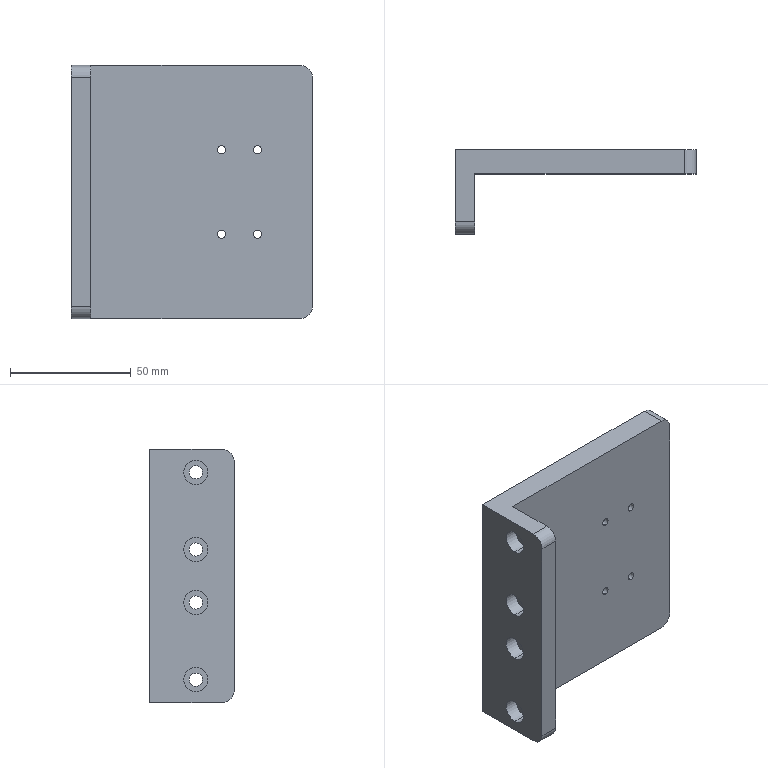Part | SolidWorks | features ICE 5, 3DProfileFeature 2, Fillet 2, HoleWzd 2, ExtruThin 1 | 1 solid | 40 faces | box 100 x 35 x 105 mm | volume 123455 mm3 | cylinder 28 | plane 12 | commonest cylinder face diameters 10 x12 3.3 x8 5.5 x8
STEP:
#1=CARTESIAN_POINT('',(-4.3,-19.1,-48.));
#2=VERTEX_POINT('',#1);
#3=CARTESIAN_POINT('',(-4.3,-19.1,-38.));
#4=VERTEX_POINT('',#3);
#5=CARTESIAN_POINT('',(-4.3,-19.1,-43.));
#6=DIRECTION('',(-1.,0.,0.));
#7=DIRECTION('',(0.,0.,1.));
#8=AXIS2_PLACEMENT_3D('',#5,#6,#7);
#9=CIRCLE('',#8,5.);
#10=EDGE_CURVE('',#2,#4,#9,.T.);
#11=ORIENTED_EDGE('',*,*,#10,.F.);
#12=CARTESIAN_POINT('',(-10.,-19.1,-48.));
#13=VERTEX_POINT('',#12);
#14=CARTESIAN_POINT('',(-10.,-19.1,-48.));
#15=DIRECTION('',(-1.,0.,0.));
#16=VECTOR('',#15,1000.);
#17=LINE('',#14,#16);
#18=EDGE_CURVE('',#2,#13,#17,.T.);
#19=ORIENTED_EDGE('',*,*,#18,.T.);
#20=CARTESIAN_POINT('',(-10.,-19.1,-38.));
#21=VERTEX_POINT('',#20);
#22=CARTESIAN_POINT('',(-10.,-19.1,-43.));
#23=DIRECTION('',(-1.,0.,0.));
#24=DIRECTION('',(0.,0.,1.));
#25=AXIS2_PLACEMENT_3D('',#22,#23,#24);
#26=CIRCLE('',#25,5.);
#27=EDGE_CURVE('',#13,#21,#26,.T.);
#28=ORIENTED_EDGE('',*,*,#27,.T.);
#29=CARTESIAN_POINT('',(-10.,-19.1,-38.));
#30=DIRECTION('',(-1.,0.,0.));
#31=VECTOR('',#30,1000.);
#32=LINE('',#29,#31);
#33=EDGE_CURVE('',#4,#21,#32,.T.);
#34=ORIENTED_EDGE('',*,*,#33,.F.);
#35=EDGE_LOOP('',(#11,#19,#28,#34));
#36=FACE_OUTER_BOUND('',#35,.T.);
#37=CARTESIAN_POINT('',(-10.,-19.1,-43.));
#38=DIRECTION('',(-1.,0.,0.));
#39=DIRECTION('',(0.,0.,1.));
#40=AXIS2_PLACEMENT_3D('',#37,#38,#39);
#41=CYLINDRICAL_SURFACE('',#40,5.);
#42=ADVANCED_FACE('',(#36),#41,.F.);
#43=CARTESIAN_POINT('',(-2.,-19.1,-45.75));
#44=VERTEX_POINT('',#43);
#45=CARTESIAN_POINT('',(-2.,-19.1,-40.25));
#46=VERTEX_POINT('',#45);
#47=CARTESIAN_POINT('',(-2.,-19.1,-43.));
#48=DIRECTION('',(-1.,0.,0.));
#49=DIRECTION('',(0.,0.,1.));
#50=AXIS2_PLACEMENT_3D('',#47,#48,#49);
#51=CIRCLE('',#50,2.75);
#52=EDGE_CURVE('',#44,#46,#51,.T.);
#53=ORIENTED_EDGE('',*,*,#52,.F.);
#54=CARTESIAN_POINT('',(-4.3,-19.1,-45.75));
#55=VERTEX_POINT('',#54);
#56=CARTESIAN_POINT('',(-10.,-19.1,-45.75));
#57=DIRECTION('',(-1.,0.,0.));
#58=VECTOR('',#57,1000.);
#59=LINE('',#56,#58);
#60=EDGE_CURVE('',#44,#55,#59,.T.);
#61=ORIENTED_EDGE('',*,*,#60,.T.);
#62=CARTESIAN_POINT('',(-4.3,-19.1,-40.25));
#63=VERTEX_POINT('',#62);
#64=CARTESIAN_POINT('',(-4.3,-19.1,-43.));
#65=DIRECTION('',(-1.,0.,0.));
#66=DIRECTION('',(0.,0.,1.));
#67=AXIS2_PLACEMENT_3D('',#64,#65,#66);
#68=CIRCLE('',#67,2.75);
#69=EDGE_CURVE('',#55,#63,#68,.T.);
#70=ORIENTED_EDGE('',*,*,#69,.T.);
#71=CARTESIAN_POINT('',(-10.,-19.1,-40.25));
#72=DIRECTION('',(-1.,0.,0.));
#73=VECTOR('',#72,1000.);
#74=LINE('',#71,#73);
#75=EDGE_CURVE('',#46,#63,#74,.T.);
#76=ORIENTED_EDGE('',*,*,#75,.F.);
#77=EDGE_LOOP('',(#53,#61,#70,#76));
#78=FACE_OUTER_BOUND('',#77,.T.);
#79=CARTESIAN_POINT('',(-10.,-19.1,-43.));
#80=DIRECTION('',(-1.,0.,0.));
#81=DIRECTION('',(0.,0.,1.));
#82=AXIS2_PLACEMENT_3D('',#79,#80,#81);
#83=CYLINDRICAL_SURFACE('',#82,2.75);
#84=ADVANCED_FACE('',(#78),#83,.F.);
#85=CARTESIAN_POINT('',(-4.3,-19.1,-16.));
#86=VERTEX_POINT('',#85);
#87=CARTESIAN_POINT('',(-4.3,-19.1,-6.));
#88=VERTEX_POINT('',#87);
#89=CARTESIAN_POINT('',(-4.3,-19.1,-11.));
#90=DIRECTION('',(-1.,0.,0.));
#91=DIRECTION('',(0.,0.,1.));
#92=AXIS2_PLACEMENT_3D('',#89,#90,#91);
#93=CIRCLE('',#92,5.);
#94=EDGE_CURVE('',#86,#88,#93,.T.);
#95=ORIENTED_EDGE('',*,*,#94,.F.);
#96=CARTESIAN_POINT('',(-10.,-19.1,-16.));
#97=VERTEX_POINT('',#96);
#98=CARTESIAN_POINT('',(-10.,-19.1,-16.));
#99=DIRECTION('',(-1.,0.,0.));
#100=VECTOR('',#99,1000.);
#101=LINE('',#98,#100);
#102=EDGE_CURVE('',#86,#97,#101,.T.);
#103=ORIENTED_EDGE('',*,*,#102,.T.);
#104=CARTESIAN_POINT('',(-10.,-19.1,-6.));
#105=VERTEX_POINT('',#104);
#106=CARTESIAN_POINT('',(-10.,-19.1,-11.));
#107=DIRECTION('',(-1.,0.,0.));
#108=DIRECTION('',(0.,0.,1.));
#109=AXIS2_PLACEMENT_3D('',#106,#107,#108);
#110=CIRCLE('',#109,5.);
#111=EDGE_CURVE('',#97,#105,#110,.T.);
#112=ORIENTED_EDGE('',*,*,#111,.T.);
#113=CARTESIAN_POINT('',(-10.,-19.1,-6.));
#114=DIRECTION('',(-1.,0.,0.));
#115=VECTOR('',#114,1000.);
#116=LINE('',#113,#115);
#117=EDGE_CURVE('',#88,#105,#116,.T.);
#118=ORIENTED_EDGE('',*,*,#117,.F.);
#119=EDGE_LOOP('',(#95,#103,#112,#118));
#120=FACE_OUTER_BOUND('',#119,.T.);
#121=CARTESIAN_POINT('',(-10.,-19.1,-11.));
#122=DIRECTION('',(-1.,0.,0.));
#123=DIRECTION('',(0.,0.,1.));
#124=AXIS2_PLACEMENT_3D('',#121,#122,#123);
#125=CYLINDRICAL_SURFACE('',#124,5.);
#126=ADVANCED_FACE('',(#120),#125,.F.);
#127=CARTESIAN_POINT('',(-2.,-19.1,-13.75));
#128=VERTEX_POINT('',#127);
#129=CARTESIAN_POINT('',(-2.,-19.1,-8.25));
#130=VERTEX_POINT('',#129);
#131=CARTESIAN_POINT('',(-2.,-19.1,-11.));
#132=DIRECTION('',(-1.,0.,0.));
#133=DIRECTION('',(0.,0.,1.));
#134=AXIS2_PLACEMENT_3D('',#131,#132,#133);
#135=CIRCLE('',#134,2.75);
#136=EDGE_CURVE('',#128,#130,#135,.T.);
#137=ORIENTED_EDGE('',*,*,#136,.F.);
#138=CARTESIAN_POINT('',(-4.3,-19.1,-13.75));
#139=VERTEX_POINT('',#138);
#140=CARTESIAN_POINT('',(-10.,-19.1,-13.75));
#141=DIRECTION('',(-1.,0.,0.));
#142=VECTOR('',#141,1000.);
#143=LINE('',#140,#142);
#144=EDGE_CURVE('',#128,#139,#143,.T.);
#145=ORIENTED_EDGE('',*,*,#144,.T.);
#146=CARTESIAN_POINT('',(-4.3,-19.1,-8.25));
#147=VERTEX_POINT('',#146);
#148=CARTESIAN_POINT('',(-4.3,-19.1,-11.));
#149=DIRECTION('',(-1.,0.,0.));
#150=DIRECTION('',(0.,0.,1.));
#151=AXIS2_PLACEMENT_3D('',#148,#149,#150);
#152=CIRCLE('',#151,2.75);
#153=EDGE_CURVE('',#139,#147,#152,.T.);
#154=ORIENTED_EDGE('',*,*,#153,.T.);
#155=CARTESIAN_POINT('',(-10.,-19.1,-8.25));
#156=DIRECTION('',(-1.,0.,0.));
#157=VECTOR('',#156,1000.);
#158=LINE('',#155,#157);
#159=EDGE_CURVE('',#130,#147,#158,.T.);
#160=ORIENTED_EDGE('',*,*,#159,.F.);
#161=EDGE_LOOP('',(#137,#145,#154,#160));
#162=FACE_OUTER_BOUND('',#161,.T.);
#163=CARTESIAN_POINT('',(-10.,-19.1,-11.));
#164=DIRECTION('',(-1.,0.,0.));
#165=DIRECTION('',(0.,0.,1.));
#166=AXIS2_PLACEMENT_3D('',#163,#164,#165);
#167=CYLINDRICAL_SURFACE('',#166,2.75);
#168=ADVANCED_FACE('',(#162),#167,.F.);
#169=CARTESIAN_POINT('',(-4.3,-19.1,6.));
#170=VERTEX_POINT('',#169);
#171=CARTESIAN_POINT('',(-4.3,-19.1,16.));
#172=VERTEX_POINT('',#171);
#173=CARTESIAN_POINT('',(-4.3,-19.1,11.));
#174=DIRECTION('',(-1.,0.,0.));
#175=DIRECTION('',(0.,0.,1.));
#176=AXIS2_PLACEMENT_3D('',#173,#174,#175);
#177=CIRCLE('',#176,5.);
#178=EDGE_CURVE('',#170,#172,#177,.T.);
#179=ORIENTED_EDGE('',*,*,#178,.F.);
#180=CARTESIAN_POINT('',(-10.,-19.1,6.));
#181=VERTEX_POINT('',#180);
#182=CARTESIAN_POINT('',(-10.,-19.1,6.));
#183=DIRECTION('',(-1.,0.,0.));
#184=VECTOR('',#183,1000.);
#185=LINE('',#182,#184);
#186=EDGE_CURVE('',#170,#181,#185,.T.);
#187=ORIENTED_EDGE('',*,*,#186,.T.);
#188=CARTESIAN_POINT('',(-10.,-19.1,16.));
#189=VERTEX_POINT('',#188);
#190=CARTESIAN_POINT('',(-10.,-19.1,11.));
#191=DIRECTION('',(-1.,0.,0.));
#192=DIRECTION('',(0.,0.,1.));
#193=AXIS2_PLACEMENT_3D('',#190,#191,#192);
#194=CIRCLE('',#193,5.);
#195=EDGE_CURVE('',#181,#189,#194,.T.);
#196=ORIENTED_EDGE('',*,*,#195,.T.);
#197=CARTESIAN_POINT('',(-10.,-19.1,16.));
#198=DIRECTION('',(-1.,0.,0.));
#199=VECTOR('',#198,1000.);
#200=LINE('',#197,#199);
#201=EDGE_CURVE('',#172,#189,#200,.T.);
#202=ORIENTED_EDGE('',*,*,#201,.F.);
#203=EDGE_LOOP('',(#179,#187,#196,#202));
#204=FACE_OUTER_BOUND('',#203,.T.);
#205=CARTESIAN_POINT('',(-10.,-19.1,11.));
#206=DIRECTION('',(-1.,0.,0.));
#207=DIRECTION('',(0.,0.,1.));
#208=AXIS2_PLACEMENT_3D('',#205,#206,#207);
#209=CYLINDRICAL_SURFACE('',#208,5.);
#210=ADVANCED_FACE('',(#204),#209,.F.);
#211=CARTESIAN_POINT('',(-2.,-19.1,8.25));
#212=VERTEX_POINT('',#211);
#213=CARTESIAN_POINT('',(-2.,-19.1,13.75));
#214=VERTEX_POINT('',#213);
#215=CARTESIAN_POINT('',(-2.,-19.1,11.));
#216=DIRECTION('',(-1.,0.,0.));
#217=DIRECTION('',(0.,0.,1.));
#218=AXIS2_PLACEMENT_3D('',#215,#216,#217);
#219=CIRCLE('',#218,2.75);
#220=EDGE_CURVE('',#212,#214,#219,.T.);
#221=ORIENTED_EDGE('',*,*,#220,.F.);
#222=CARTESIAN_POINT('',(-4.3,-19.1,8.25));
#223=VERTEX_POINT('',#222);
#224=CARTESIAN_POINT('',(-10.,-19.1,8.25));
#225=DIRECTION('',(-1.,0.,0.));
#226=VECTOR('',#225,1000.);
#227=LINE('',#224,#226);
#228=EDGE_CURVE('',#212,#223,#227,.T.);
#229=ORIENTED_EDGE('',*,*,#228,.T.);
#230=CARTESIAN_POINT('',(-4.3,-19.1,13.75));
#231=VERTEX_POINT('',#230);
#232=CARTESIAN_POINT('',(-4.3,-19.1,11.));
#233=DIRECTION('',(-1.,0.,0.));
#234=DIRECTION('',(0.,0.,1.));
#235=AXIS2_PLACEMENT_3D('',#232,#233,#234);
#236=CIRCLE('',#235,2.75);
#237=EDGE_CURVE('',#223,#231,#236,.T.);
#238=ORIENTED_EDGE('',*,*,#237,.T.);
#239=CARTESIAN_POINT('',(-10.,-19.1,13.75));
#240=DIRECTION('',(-1.,0.,0.));
#241=VECTOR('',#240,1000.);
#242=LINE('',#239,#241);
#243=EDGE_CURVE('',#214,#231,#242,.T.);
#244=ORIENTED_EDGE('',*,*,#243,.F.);
#245=EDGE_LOOP('',(#221,#229,#238,#244));
#246=FACE_OUTER_BOUND('',#245,.T.);
#247=CARTESIAN_POINT('',(-10.,-19.1,11.));
#248=DIRECTION('',(-1.,0.,0.));
#249=DIRECTION('',(0.,0.,1.));
#250=AXIS2_PLACEMENT_3D('',#247,#248,#249);
#251=CYLINDRICAL_SURFACE('',#250,2.75);
#252=ADVANCED_FACE('',(#246),#251,.F.);
#253=CARTESIAN_POINT('',(-4.3,-19.1,38.));
#254=VERTEX_POINT('',#253);
#255=CARTESIAN_POINT('',(-4.3,-19.1,48.));
#256=VERTEX_POINT('',#255);
#257=CARTESIAN_POINT('',(-4.3,-19.1,43.));
#258=DIRECTION('',(-1.,0.,0.));
#259=DIRECTION('',(0.,0.,1.));
#260=AXIS2_PLACEMENT_3D('',#257,#258,#259);
#261=CIRCLE('',#260,5.);
#262=EDGE_CURVE('',#254,#256,#261,.T.);
#263=ORIENTED_EDGE('',*,*,#262,.F.);
#264=CARTESIAN_POINT('',(-10.,-19.1,38.));
#265=VERTEX_POINT('',#264);
#266=CARTESIAN_POINT('',(-10.,-19.1,38.));
#267=DIRECTION('',(-1.,0.,0.));
#268=VECTOR('',#267,1000.);
#269=LINE('',#266,#268);
#270=EDGE_CURVE('',#254,#265,#269,.T.);
#271=ORIENTED_EDGE('',*,*,#270,.T.);
#272=CARTESIAN_POINT('',(-10.,-19.1,48.));
#273=VERTEX_POINT('',#272);
#274=CARTESIAN_POINT('',(-10.,-19.1,43.));
#275=DIRECTION('',(-1.,0.,0.));
#276=DIRECTION('',(0.,0.,1.));
#277=AXIS2_PLACEMENT_3D('',#274,#275,#276);
#278=CIRCLE('',#277,5.);
#279=EDGE_CURVE('',#265,#273,#278,.T.);
#280=ORIENTED_EDGE('',*,*,#279,.T.);
#281=CARTESIAN_POINT('',(-10.,-19.1,48.));
#282=DIRECTION('',(-1.,0.,0.));
#283=VECTOR('',#282,1000.);
#284=LINE('',#281,#283);
#285=EDGE_CURVE('',#256,#273,#284,.T.);
#286=ORIENTED_EDGE('',*,*,#285,.F.);
#287=EDGE_LOOP('',(#263,#271,#280,#286));
#288=FACE_OUTER_BOUND('',#287,.T.);
#289=CARTESIAN_POINT('',(-10.,-19.1,43.));
#290=DIRECTION('',(-1.,0.,0.));
#291=DIRECTION('',(0.,0.,1.));
#292=AXIS2_PLACEMENT_3D('',#289,#290,#291);
#293=CYLINDRICAL_SURFACE('',#292,5.);
#294=ADVANCED_FACE('',(#288),#293,.F.);
#295=CARTESIAN_POINT('',(-2.,-19.1,40.25));
#296=VERTEX_POINT('',#295);
#297=CARTESIAN_POINT('',(-2.,-19.1,45.75));
#298=VERTEX_POINT('',#297);
#299=CARTESIAN_POINT('',(-2.,-19.1,43.));
#300=DIRECTION('',(-1.,0.,0.));
#301=DIRECTION('',(0.,0.,1.));
#302=AXIS2_PLACEMENT_3D('',#299,#300,#301);
#303=CIRCLE('',#302,2.75);
#304=EDGE_CURVE('',#296,#298,#303,.T.);
#305=ORIENTED_EDGE('',*,*,#304,.F.);
#306=CARTESIAN_POINT('',(-4.3,-19.1,40.25));
#307=VERTEX_POINT('',#306);
#308=CARTESIAN_POINT('',(-10.,-19.1,40.25));
#309=DIRECTION('',(-1.,0.,0.));
#310=VECTOR('',#309,1000.);
#311=LINE('',#308,#310);
#312=EDGE_CURVE('',#296,#307,#311,.T.);
#313=ORIENTED_EDGE('',*,*,#312,.T.);
#314=CARTESIAN_POINT('',(-4.3,-19.1,45.75));
#315=VERTEX_POINT('',#314);
#316=CARTESIAN_POINT('',(-4.3,-19.1,43.));
#317=DIRECTION('',(-1.,0.,0.));
#318=DIRECTION('',(0.,0.,1.));
#319=AXIS2_PLACEMENT_3D('',#316,#317,#318);
#320=CIRCLE('',#319,2.75);
#321=EDGE_CURVE('',#307,#315,#320,.T.);
#322=ORIENTED_EDGE('',*,*,#321,.T.);
#323=CARTESIAN_POINT('',(-10.,-19.1,45.75));
#324=DIRECTION('',(-1.,0.,0.));
#325=VECTOR('',#324,1000.);
#326=LINE('',#323,#325);
#327=EDGE_CURVE('',#298,#315,#326,.T.);
#328=ORIENTED_EDGE('',*,*,#327,.F.);
#329=EDGE_LOOP('',(#305,#313,#322,#328));
#330=FACE_OUTER_BOUND('',#329,.T.);
#331=CARTESIAN_POINT('',(-10.,-19.1,43.));
#332=DIRECTION('',(-1.,0.,0.));
#333=DIRECTION('',(0.,0.,1.));
#334=AXIS2_PLACEMENT_3D('',#331,#332,#333);
#335=CYLINDRICAL_SURFACE('',#334,2.75);
#336=ADVANCED_FACE('',(#330),#335,.F.);
#337=CARTESIAN_POINT('',(67.2,-10.,15.85));
#338=VERTEX_POINT('',#337);
#339=CARTESIAN_POINT('',(67.2,-10.,19.15));
#340=VERTEX_POINT('',#339);
#341=CARTESIAN_POINT('',(67.2,-10.,17.5));
#342=DIRECTION('',(0.,1.,0.));
#343=DIRECTION('',(0.,0.,1.));
#344=AXIS2_PLACEMENT_3D('',#341,#342,#343);
#345=CIRCLE('',#344,1.65);
#346=EDGE_CURVE('',#338,#340,#345,.T.);
#347=ORIENTED_EDGE('',*,*,#346,.F.);
#348=CARTESIAN_POINT('',(67.2,0.,15.85));
#349=VERTEX_POINT('',#348);
#350=CARTESIAN_POINT('',(67.2,0.,15.85));
#351=DIRECTION('',(0.,1.,0.));
#352=VECTOR('',#351,1000.);
#353=LINE('',#350,#352);
#354=EDGE_CURVE('',#338,#349,#353,.T.);
#355=ORIENTED_EDGE('',*,*,#354,.T.);
#356=CARTESIAN_POINT('',(67.2,0.,19.15));
#357=VERTEX_POINT('',#356);
#358=CARTESIAN_POINT('',(67.2,0.,17.5));
#359=DIRECTION('',(0.,1.,0.));
#360=DIRECTION('',(0.,0.,1.));
#361=AXIS2_PLACEMENT_3D('',#358,#359,#360);
#362=CIRCLE('',#361,1.65);
#363=EDGE_CURVE('',#349,#357,#362,.T.);
#364=ORIENTED_EDGE('',*,*,#363,.T.);
#365=CARTESIAN_POINT('',(67.2,0.,19.15));
#366=DIRECTION('',(0.,1.,0.));
#367=VECTOR('',#366,1000.);
#368=LINE('',#365,#367);
#369=EDGE_CURVE('',#340,#357,#368,.T.);
#370=ORIENTED_EDGE('',*,*,#369,.F.);
#371=EDGE_LOOP('',(#347,#355,#364,#370));
#372=FACE_OUTER_BOUND('',#371,.T.);
#373=CARTESIAN_POINT('',(67.2,0.,17.5));
#374=DIRECTION('',(0.,1.,0.));
#375=DIRECTION('',(0.,0.,1.));
#376=AXIS2_PLACEMENT_3D('',#373,#374,#375);
#377=CYLINDRICAL_SURFACE('',#376,1.65);
#378=ADVANCED_FACE('',(#372),#377,.F.);
#379=CARTESIAN_POINT('',(52.2,-10.,15.85));
#380=VERTEX_POINT('',#379);
#381=CARTESIAN_POINT('',(52.2,-10.,19.15));
#382=VERTEX_POINT('',#381);
#383=CARTESIAN_POINT('',(52.2,-10.,17.5));
#384=DIRECTION('',(0.,1.,0.));
#385=DIRECTION('',(0.,0.,1.));
#386=AXIS2_PLACEMENT_3D('',#383,#384,#385);
#387=CIRCLE('',#386,1.65);
#388=EDGE_CURVE('',#380,#382,#387,.T.);
#389=ORIENTED_EDGE('',*,*,#388,.F.);
#390=CARTESIAN_POINT('',(52.2,0.,15.85));
#391=VERTEX_POINT('',#390);
#392=CARTESIAN_POINT('',(52.2,0.,15.85));
#393=DIRECTION('',(0.,1.,0.));
#394=VECTOR('',#393,1000.);
#395=LINE('',#392,#394);
#396=EDGE_CURVE('',#380,#391,#395,.T.);
#397=ORIENTED_EDGE('',*,*,#396,.T.);
#398=CARTESIAN_POINT('',(52.2,0.,19.15));
#399=VERTEX_POINT('',#398);
#400=CARTESIAN_POINT('',(52.2,0.,17.5));
#401=DIRECTION('',(0.,1.,0.));
#402=DIRECTION('',(0.,0.,1.));
#403=AXIS2_PLACEMENT_3D('',#400,#401,#402);
#404=CIRCLE('',#403,1.65);
#405=EDGE_CURVE('',#391,#399,#404,.T.);
#406=ORIENTED_EDGE('',*,*,#405,.T.);
#407=CARTESIAN_POINT('',(52.2,0.,19.15));
#408=DIRECTION('',(0.,1.,0.));
#409=VECTOR('',#408,1000.);
#410=LINE('',#407,#409);
#411=EDGE_CURVE('',#382,#399,#410,.T.);
#412=ORIENTED_EDGE('',*,*,#411,.F.);
#413=EDGE_LOOP('',(#389,#397,#406,#412));
#414=FACE_OUTER_BOUND('',#413,.T.);
#415=CARTESIAN_POINT('',(52.2,0.,17.5));
#416=DIRECTION('',(0.,1.,0.));
#417=DIRECTION('',(0.,0.,1.));
#418=AXIS2_PLACEMENT_3D('',#415,#416,#417);
#419=CYLINDRICAL_SURFACE('',#418,1.65);
#420=ADVANCED_FACE('',(#414),#419,.F.);
#421=CARTESIAN_POINT('',(67.2,-10.,-19.15));
#422=VERTEX_POINT('',#421);
#423=CARTESIAN_POINT('',(67.2,-10.,-15.85));
#424=VERTEX_POINT('',#423);
#425=CARTESIAN_POINT('',(67.2,-10.,-17.5));
#426=DIRECTION('',(0.,1.,0.));
#427=DIRECTION('',(0.,0.,1.));
#428=AXIS2_PLACEMENT_3D('',#425,#426,#427);
#429=CIRCLE('',#428,1.65);
#430=EDGE_CURVE('',#422,#424,#429,.T.);
#431=ORIENTED_EDGE('',*,*,#430,.F.);
#432=CARTESIAN_POINT('',(67.2,0.,-19.15));
#433=VERTEX_POINT('',#432);
#434=CARTESIAN_POINT('',(67.2,0.,-19.15));
#435=DIRECTION('',(0.,1.,0.));
#436=VECTOR('',#435,1000.);
#437=LINE('',#434,#436);
#438=EDGE_CURVE('',#422,#433,#437,.T.);
#439=ORIENTED_EDGE('',*,*,#438,.T.);
#440=CARTESIAN_POINT('',(67.2,0.,-15.85));
#441=VERTEX_POINT('',#440);
#442=CARTESIAN_POINT('',(67.2,0.,-17.5));
#443=DIRECTION('',(0.,1.,0.));
#444=DIRECTION('',(0.,0.,1.));
#445=AXIS2_PLACEMENT_3D('',#442,#443,#444);
#446=CIRCLE('',#445,1.65);
#447=EDGE_CURVE('',#433,#441,#446,.T.);
#448=ORIENTED_EDGE('',*,*,#447,.T.);
#449=CARTESIAN_POINT('',(67.2,0.,-15.85));
#450=DIRECTION('',(0.,1.,0.));
#451=VECTOR('',#450,1000.);
#452=LINE('',#449,#451);
#453=EDGE_CURVE('',#424,#441,#452,.T.);
#454=ORIENTED_EDGE('',*,*,#453,.F.);
#455=EDGE_LOOP('',(#431,#439,#448,#454));
#456=FACE_OUTER_BOUND('',#455,.T.);
#457=CARTESIAN_POINT('',(67.2,0.,-17.5));
#458=DIRECTION('',(0.,1.,0.));
#459=DIRECTION('',(0.,0.,1.));
#460=AXIS2_PLACEMENT_3D('',#457,#458,#459);
#461=CYLINDRICAL_SURFACE('',#460,1.65);
#462=ADVANCED_FACE('',(#456),#461,.F.);
#463=CARTESIAN_POINT('',(52.2,-10.,-19.15));
#464=VERTEX_POINT('',#463);
#465=CARTESIAN_POINT('',(52.2,-10.,-15.85));
#466=VERTEX_POINT('',#465);
#467=CARTESIAN_POINT('',(52.2,-10.,-17.5));
#468=DIRECTION('',(0.,1.,0.));
#469=DIRECTION('',(0.,0.,1.));
#470=AXIS2_PLACEMENT_3D('',#467,#468,#469);
#471=CIRCLE('',#470,1.65);
#472=EDGE_CURVE('',#464,#466,#471,.T.);
#473=ORIENTED_EDGE('',*,*,#472,.F.);
#474=CARTESIAN_POINT('',(52.2,0.,-19.15));
#475=VERTEX_POINT('',#474);
#476=CARTESIAN_POINT('',(52.2,0.,-19.15));
#477=DIRECTION('',(0.,1.,0.));
#478=VECTOR('',#477,1000.);
#479=LINE('',#476,#478);
#480=EDGE_CURVE('',#464,#475,#479,.T.);
#481=ORIENTED_EDGE('',*,*,#480,.T.);
#482=CARTESIAN_POINT('',(52.2,0.,-15.85));
#483=VERTEX_POINT('',#482);
#484=CARTESIAN_POINT('',(52.2,0.,-17.5));
#485=DIRECTION('',(0.,1.,0.));
#486=DIRECTION('',(0.,0.,1.));
#487=AXIS2_PLACEMENT_3D('',#484,#485,#486);
#488=CIRCLE('',#487,1.65);
#489=EDGE_CURVE('',#475,#483,#488,.T.);
#490=ORIENTED_EDGE('',*,*,#489,.T.);
#491=CARTESIAN_POINT('',(52.2,0.,-15.85));
#492=DIRECTION('',(0.,1.,0.));
#493=VECTOR('',#492,1000.);
#494=LINE('',#491,#493);
#495=EDGE_CURVE('',#466,#483,#494,.T.);
#496=ORIENTED_EDGE('',*,*,#495,.F.);
#497=EDGE_LOOP('',(#473,#481,#490,#496));
#498=FACE_OUTER_BOUND('',#497,.T.);
#499=CARTESIAN_POINT('',(52.2,0.,-17.5));
#500=DIRECTION('',(0.,1.,0.));
#501=DIRECTION('',(0.,0.,1.));
#502=AXIS2_PLACEMENT_3D('',#499,#500,#501);
#503=CYLINDRICAL_SURFACE('',#502,1.65);
#504=ADVANCED_FACE('',(#498),#503,.F.);
#505=CARTESIAN_POINT('',(-10.,-19.1,-11.));
#506=DIRECTION('',(-1.,0.,0.));
#507=DIRECTION('',(0.,0.,1.));
#508=AXIS2_PLACEMENT_3D('',#505,#506,#507);
#509=CIRCLE('',#508,5.);
#510=EDGE_CURVE('',#105,#97,#509,.T.);
#511=ORIENTED_EDGE('',*,*,#510,.F.);
#512=ORIENTED_EDGE('',*,*,#111,.F.);
#513=EDGE_LOOP('',(#511,#512));
#514=FACE_BOUND('',#513,.T.);
#515=CARTESIAN_POINT('',(-10.,-19.1,11.));
#516=DIRECTION('',(-1.,0.,0.));
#517=DIRECTION('',(0.,0.,1.));
#518=AXIS2_PLACEMENT_3D('',#515,#516,#517);
#519=CIRCLE('',#518,5.);
#520=EDGE_CURVE('',#189,#181,#519,.T.);
#521=ORIENTED_EDGE('',*,*,#520,.F.);
#522=ORIENTED_EDGE('',*,*,#195,.F.);
#523=EDGE_LOOP('',(#521,#522));
#524=FACE_BOUND('',#523,.T.);
#525=CARTESIAN_POINT('',(-10.,-19.1,43.));
#526=DIRECTION('',(-1.,0.,0.));
#527=DIRECTION('',(0.,0.,1.));
#528=AXIS2_PLACEMENT_3D('',#525,#526,#527);
#529=CIRCLE('',#528,5.);
#530=EDGE_CURVE('',#273,#265,#529,.T.);
#531=ORIENTED_EDGE('',*,*,#530,.F.);
#532=ORIENTED_EDGE('',*,*,#279,.F.);
#533=EDGE_LOOP('',(#531,#532));
#534=FACE_BOUND('',#533,.T.);
#535=CARTESIAN_POINT('',(-10.,-30.,-52.5));
#536=VERTEX_POINT('',#535);
#537=CARTESIAN_POINT('',(-10.,0.,-52.5));
#538=VERTEX_POINT('',#537);
#539=CARTESIAN_POINT('',(-10.,-155.,-52.5));
#540=DIRECTION('',(0.,1.,0.));
#541=VECTOR('',#540,1000.);
#542=LINE('',#539,#541);
#543=EDGE_CURVE('',#536,#538,#542,.T.);
#544=ORIENTED_EDGE('',*,*,#543,.F.);
#545=CARTESIAN_POINT('',(-10.,-35.,-47.5));
#546=VERTEX_POINT('',#545);
#547=CARTESIAN_POINT('',(-10.,-30.,-47.5));
#548=DIRECTION('',(-1.,0.,0.));
#549=DIRECTION('',(0.,0.,-1.));
#550=AXIS2_PLACEMENT_3D('',#547,#548,#549);
#551=CIRCLE('',#550,5.);
#552=EDGE_CURVE('',#536,#546,#551,.T.);
#553=ORIENTED_EDGE('',*,*,#552,.T.);
#554=CARTESIAN_POINT('',(-10.,-35.,47.5));
#555=VERTEX_POINT('',#554);
#556=CARTESIAN_POINT('',(-10.,-35.,-52.5));
#557=DIRECTION('',(0.,0.,1.));
#558=VECTOR('',#557,1000.);
#559=LINE('',#556,#558);
#560=EDGE_CURVE('',#546,#555,#559,.T.);
#561=ORIENTED_EDGE('',*,*,#560,.T.);
#562=CARTESIAN_POINT('',(-10.,-30.,52.5));
#563=VERTEX_POINT('',#562);
#564=CARTESIAN_POINT('',(-10.,-30.,47.5));
#565=DIRECTION('',(-1.,0.,0.));
#566=DIRECTION('',(0.,0.,-1.));
#567=AXIS2_PLACEMENT_3D('',#564,#565,#566);
#568=CIRCLE('',#567,5.);
#569=EDGE_CURVE('',#555,#563,#568,.T.);
#570=ORIENTED_EDGE('',*,*,#569,.T.);
#571=CARTESIAN_POINT('',(-10.,0.,52.5));
#572=VERTEX_POINT('',#571);
#573=CARTESIAN_POINT('',(-10.,-155.,52.5));
#574=DIRECTION('',(0.,1.,0.));
#575=VECTOR('',#574,1000.);
#576=LINE('',#573,#575);
#577=EDGE_CURVE('',#563,#572,#576,.T.);
#578=ORIENTED_EDGE('',*,*,#577,.T.);
#579=CARTESIAN_POINT('',(-10.,0.,52.5));
#580=DIRECTION('',(0.,0.,1.));
#581=VECTOR('',#580,1000.);
#582=LINE('',#579,#581);
#583=EDGE_CURVE('',#538,#572,#582,.T.);
#584=ORIENTED_EDGE('',*,*,#583,.F.);
#585=EDGE_LOOP('',(#544,#553,#561,#570,#578,#584));
#586=FACE_OUTER_BOUND('',#585,.T.);
#587=CARTESIAN_POINT('',(-10.,-19.1,-43.));
#588=DIRECTION('',(-1.,0.,0.));
#589=DIRECTION('',(0.,0.,1.));
#590=AXIS2_PLACEMENT_3D('',#587,#588,#589);
#591=CIRCLE('',#590,5.);
#592=EDGE_CURVE('',#21,#13,#591,.T.);
#593=ORIENTED_EDGE('',*,*,#592,.F.);
#594=ORIENTED_EDGE('',*,*,#27,.F.);
#595=EDGE_LOOP('',(#593,#594));
#596=FACE_BOUND('',#595,.T.);
#597=CARTESIAN_POINT('',(-10.,0.,27.));
#598=DIRECTION('',(1.,0.,0.));
#599=DIRECTION('',(0.,0.,-1.));
#600=AXIS2_PLACEMENT_3D('',#597,#598,#599);
#601=PLANE('',#600);
#602=ADVANCED_FACE('',(#514,#524,#534,#586,#596),#601,.F.);
#603=CARTESIAN_POINT('',(52.2,-10.,-17.5));
#604=DIRECTION('',(0.,1.,0.));
#605=DIRECTION('',(0.,0.,1.));
#606=AXIS2_PLACEMENT_3D('',#603,#604,#605);
#607=CIRCLE('',#606,1.65);
#608=EDGE_CURVE('',#466,#464,#607,.T.);
#609=ORIENTED_EDGE('',*,*,#608,.T.);
#610=ORIENTED_EDGE('',*,*,#472,.T.);
#611=EDGE_LOOP('',(#609,#610));
#612=FACE_BOUND('',#611,.T.);
#613=CARTESIAN_POINT('',(67.2,-10.,-17.5));
#614=DIRECTION('',(0.,1.,0.));
#615=DIRECTION('',(0.,0.,1.));
#616=AXIS2_PLACEMENT_3D('',#613,#614,#615);
#617=CIRCLE('',#616,1.65);
#618=EDGE_CURVE('',#424,#422,#617,.T.);
#619=ORIENTED_EDGE('',*,*,#618,.T.);
#620=ORIENTED_EDGE('',*,*,#430,.T.);
#621=EDGE_LOOP('',(#619,#620));
#622=FACE_BOUND('',#621,.T.);
#623=CARTESIAN_POINT('',(52.2,-10.,17.5));
#624=DIRECTION('',(0.,1.,0.));
#625=DIRECTION('',(0.,0.,1.));
#626=AXIS2_PLACEMENT_3D('',#623,#624,#625);
#627=CIRCLE('',#626,1.65);
#628=EDGE_CURVE('',#382,#380,#627,.T.);
#629=ORIENTED_EDGE('',*,*,#628,.T.);
#630=ORIENTED_EDGE('',*,*,#388,.T.);
#631=EDGE_LOOP('',(#629,#630));
#632=FACE_BOUND('',#631,.T.);
#633=CARTESIAN_POINT('',(67.2,-10.,17.5));
#634=DIRECTION('',(0.,1.,0.));
#635=DIRECTION('',(0.,0.,1.));
#636=AXIS2_PLACEMENT_3D('',#633,#634,#635);
#637=CIRCLE('',#636,1.65);
#638=EDGE_CURVE('',#340,#338,#637,.T.);
#639=ORIENTED_EDGE('',*,*,#638,.T.);
#640=ORIENTED_EDGE('',*,*,#346,.T.);
#641=EDGE_LOOP('',(#639,#640));
#642=FACE_BOUND('',#641,.T.);
#643=CARTESIAN_POINT('',(-2.,-10.,-52.5));
#644=VERTEX_POINT('',#643);
#645=CARTESIAN_POINT('',(-2.,-10.,52.5));
#646=VERTEX_POINT('',#645);
#647=CARTESIAN_POINT('',(-2.,-10.,27.));
#648=DIRECTION('',(0.,0.,1.));
#649=VECTOR('',#648,1000.);
#650=LINE('',#647,#649);
#651=EDGE_CURVE('',#644,#646,#650,.T.);
#652=ORIENTED_EDGE('',*,*,#651,.F.);
#653=CARTESIAN_POINT('',(85.,-10.,-52.5));
#654=VERTEX_POINT('',#653);
#655=CARTESIAN_POINT('',(-10.,-10.,-52.5));
#656=DIRECTION('',(1.,0.,0.));
#657=VECTOR('',#656,1000.);
#658=LINE('',#655,#657);
#659=EDGE_CURVE('',#644,#654,#658,.T.);
#660=ORIENTED_EDGE('',*,*,#659,.T.);
#661=CARTESIAN_POINT('',(90.,-10.,-47.5));
#662=VERTEX_POINT('',#661);
#663=CARTESIAN_POINT('',(85.,-10.,-47.5));
#664=DIRECTION('',(0.,-1.,0.));
#665=DIRECTION('',(0.,0.,1.));
#666=AXIS2_PLACEMENT_3D('',#663,#664,#665);
#667=CIRCLE('',#666,5.);
#668=EDGE_CURVE('',#654,#662,#667,.T.);
#669=ORIENTED_EDGE('',*,*,#668,.T.);
#670=CARTESIAN_POINT('',(90.,-10.,47.5));
#671=VERTEX_POINT('',#670);
#672=CARTESIAN_POINT('',(90.,-10.,27.));
#673=DIRECTION('',(0.,0.,-1.));
#674=VECTOR('',#673,1000.);
#675=LINE('',#672,#674);
#676=EDGE_CURVE('',#671,#662,#675,.T.);
#677=ORIENTED_EDGE('',*,*,#676,.F.);
#678=CARTESIAN_POINT('',(85.,-10.,52.5));
#679=VERTEX_POINT('',#678);
#680=CARTESIAN_POINT('',(85.,-10.,47.5));
#681=DIRECTION('',(0.,-1.,0.));
#682=DIRECTION('',(0.,0.,1.));
#683=AXIS2_PLACEMENT_3D('',#680,#681,#682);
#684=CIRCLE('',#683,5.);
#685=EDGE_CURVE('',#671,#679,#684,.T.);
#686=ORIENTED_EDGE('',*,*,#685,.T.);
#687=CARTESIAN_POINT('',(-10.,-10.,52.5));
#688=DIRECTION('',(-1.,0.,0.));
#689=VECTOR('',#688,1000.);
#690=LINE('',#687,#689);
#691=EDGE_CURVE('',#679,#646,#690,.T.);
#692=ORIENTED_EDGE('',*,*,#691,.T.);
#693=EDGE_LOOP('',(#652,#660,#669,#677,#686,#692));
#694=FACE_OUTER_BOUND('',#693,.T.);
#695=CARTESIAN_POINT('',(0.,-10.,27.));
#696=DIRECTION('',(0.,1.,0.));
#697=DIRECTION('',(0.,0.,1.));
#698=AXIS2_PLACEMENT_3D('',#695,#696,#697);
#699=PLANE('',#698);
#700=ADVANCED_FACE('',(#612,#622,#632,#642,#694),#699,.F.);
#701=ORIENTED_EDGE('',*,*,#676,.T.);
#702=CARTESIAN_POINT('',(90.,0.,-47.5));
#703=VERTEX_POINT('',#702);
#704=CARTESIAN_POINT('',(90.,0.,-47.5));
#705=DIRECTION('',(0.,1.,0.));
#706=VECTOR('',#705,1000.);
#707=LINE('',#704,#706);
#708=EDGE_CURVE('',#662,#703,#707,.T.);
#709=ORIENTED_EDGE('',*,*,#708,.T.);
#710=CARTESIAN_POINT('',(90.,0.,47.5));
#711=VERTEX_POINT('',#710);
#712=CARTESIAN_POINT('',(90.,0.,27.));
#713=DIRECTION('',(0.,0.,-1.));
#714=VECTOR('',#713,1000.);
#715=LINE('',#712,#714);
#716=EDGE_CURVE('',#711,#703,#715,.T.);
#717=ORIENTED_EDGE('',*,*,#716,.F.);
#718=CARTESIAN_POINT('',(90.,0.,47.5));
#719=DIRECTION('',(0.,-1.,0.));
#720=VECTOR('',#719,1000.);
#721=LINE('',#718,#720);
#722=EDGE_CURVE('',#711,#671,#721,.T.);
#723=ORIENTED_EDGE('',*,*,#722,.T.);
#724=EDGE_LOOP('',(#701,#709,#717,#723));
#725=FACE_OUTER_BOUND('',#724,.T.);
#726=CARTESIAN_POINT('',(90.,0.,27.));
#727=DIRECTION('',(1.,0.,0.));
#728=DIRECTION('',(0.,0.,-1.));
#729=AXIS2_PLACEMENT_3D('',#726,#727,#728);
#730=PLANE('',#729);
#731=ADVANCED_FACE('',(#725),#730,.T.);
#732=CARTESIAN_POINT('',(85.,0.,52.5));
#733=VERTEX_POINT('',#732);
#734=CARTESIAN_POINT('',(-10.,0.,52.5));
#735=DIRECTION('',(1.,0.,0.));
#736=VECTOR('',#735,1000.);
#737=LINE('',#734,#736);
#738=EDGE_CURVE('',#572,#733,#737,.T.);
#739=ORIENTED_EDGE('',*,*,#738,.T.);
#740=CARTESIAN_POINT('',(85.,0.,47.5));
#741=DIRECTION('',(0.,1.,0.));
#742=DIRECTION('',(0.,0.,1.));
#743=AXIS2_PLACEMENT_3D('',#740,#741,#742);
#744=CIRCLE('',#743,5.);
#745=EDGE_CURVE('',#733,#711,#744,.T.);
#746=ORIENTED_EDGE('',*,*,#745,.T.);
#747=ORIENTED_EDGE('',*,*,#716,.T.);
#748=CARTESIAN_POINT('',(85.,0.,-52.5));
#749=VERTEX_POINT('',#748);
#750=CARTESIAN_POINT('',(85.,0.,-47.5));
#751=DIRECTION('',(0.,1.,0.));
#752=DIRECTION('',(0.,0.,1.));
#753=AXIS2_PLACEMENT_3D('',#750,#751,#752);
#754=CIRCLE('',#753,5.);
#755=EDGE_CURVE('',#703,#749,#754,.T.);
#756=ORIENTED_EDGE('',*,*,#755,.T.);
#757=CARTESIAN_POINT('',(-10.,0.,-52.5));
#758=DIRECTION('',(-1.,0.,0.));
#759=VECTOR('',#758,1000.);
#760=LINE('',#757,#759);
#761=EDGE_CURVE('',#749,#538,#760,.T.);
#762=ORIENTED_EDGE('',*,*,#761,.T.);
#763=ORIENTED_EDGE('',*,*,#583,.T.);
#764=EDGE_LOOP('',(#739,#746,#747,#756,#762,#763));
#765=FACE_OUTER_BOUND('',#764,.T.);
#766=CARTESIAN_POINT('',(67.2,0.,17.5));
#767=DIRECTION('',(0.,1.,0.));
#768=DIRECTION('',(0.,0.,1.));
#769=AXIS2_PLACEMENT_3D('',#766,#767,#768);
#770=CIRCLE('',#769,1.65);
#771=EDGE_CURVE('',#357,#349,#770,.T.);
#772=ORIENTED_EDGE('',*,*,#771,.F.);
#773=ORIENTED_EDGE('',*,*,#363,.F.);
#774=EDGE_LOOP('',(#772,#773));
#775=FACE_BOUND('',#774,.T.);
#776=CARTESIAN_POINT('',(52.2,0.,17.5));
#777=DIRECTION('',(0.,1.,0.));
#778=DIRECTION('',(0.,0.,1.));
#779=AXIS2_PLACEMENT_3D('',#776,#777,#778);
#780=CIRCLE('',#779,1.65);
#781=EDGE_CURVE('',#399,#391,#780,.T.);
#782=ORIENTED_EDGE('',*,*,#781,.F.);
#783=ORIENTED_EDGE('',*,*,#405,.F.);
#784=EDGE_LOOP('',(#782,#783));
#785=FACE_BOUND('',#784,.T.);
#786=CARTESIAN_POINT('',(67.2,0.,-17.5));
#787=DIRECTION('',(0.,1.,0.));
#788=DIRECTION('',(0.,0.,1.));
#789=AXIS2_PLACEMENT_3D('',#786,#787,#788);
#790=CIRCLE('',#789,1.65);
#791=EDGE_CURVE('',#441,#433,#790,.T.);
#792=ORIENTED_EDGE('',*,*,#791,.F.);
#793=ORIENTED_EDGE('',*,*,#447,.F.);
#794=EDGE_LOOP('',(#792,#793));
#795=FACE_BOUND('',#794,.T.);
#796=CARTESIAN_POINT('',(52.2,0.,-17.5));
#797=DIRECTION('',(0.,1.,0.));
#798=DIRECTION('',(0.,0.,1.));
#799=AXIS2_PLACEMENT_3D('',#796,#797,#798);
#800=CIRCLE('',#799,1.65);
#801=EDGE_CURVE('',#483,#475,#800,.T.);
#802=ORIENTED_EDGE('',*,*,#801,.F.);
#803=ORIENTED_EDGE('',*,*,#489,.F.);
#804=EDGE_LOOP('',(#802,#803));
#805=FACE_BOUND('',#804,.T.);
#806=CARTESIAN_POINT('',(0.,0.,27.));
#807=DIRECTION('',(0.,1.,0.));
#808=DIRECTION('',(0.,0.,1.));
#809=AXIS2_PLACEMENT_3D('',#806,#807,#808);
#810=PLANE('',#809);
#811=ADVANCED_FACE('',(#765,#775,#785,#795,#805),#810,.T.);
#812=CARTESIAN_POINT('',(-2.,-30.,-52.5));
#813=VERTEX_POINT('',#812);
#814=CARTESIAN_POINT('',(-2.,0.,-52.5));
#815=DIRECTION('',(0.,-1.,0.));
#816=VECTOR('',#815,1000.);
#817=LINE('',#814,#816);
#818=EDGE_CURVE('',#644,#813,#817,.T.);
#819=ORIENTED_EDGE('',*,*,#818,.T.);
#820=CARTESIAN_POINT('',(-10.,-30.,-52.5));
#821=DIRECTION('',(-1.,0.,0.));
#822=VECTOR('',#821,1000.);
#823=LINE('',#820,#822);
#824=EDGE_CURVE('',#813,#536,#823,.T.);
#825=ORIENTED_EDGE('',*,*,#824,.T.);
#826=ORIENTED_EDGE('',*,*,#543,.T.);
#827=ORIENTED_EDGE('',*,*,#761,.F.);
#828=CARTESIAN_POINT('',(85.,-155.,-52.5));
#829=DIRECTION('',(0.,-1.,0.));
#830=VECTOR('',#829,1000.);
#831=LINE('',#828,#830);
#832=EDGE_CURVE('',#749,#654,#831,.T.);
#833=ORIENTED_EDGE('',*,*,#832,.T.);
#834=ORIENTED_EDGE('',*,*,#659,.F.);
#835=EDGE_LOOP('',(#819,#825,#826,#827,#833,#834));
#836=FACE_OUTER_BOUND('',#835,.T.);
#837=CARTESIAN_POINT('',(-10.,-155.,-52.5));
#838=DIRECTION('',(0.,0.,-1.));
#839=DIRECTION('',(-1.,0.,0.));
#840=AXIS2_PLACEMENT_3D('',#837,#838,#839);
#841=PLANE('',#840);
#842=ADVANCED_FACE('',(#836),#841,.T.);
#843=ORIENTED_EDGE('',*,*,#577,.F.);
#844=CARTESIAN_POINT('',(-2.,-30.,52.5));
#845=VERTEX_POINT('',#844);
#846=CARTESIAN_POINT('',(-10.,-30.,52.5));
#847=DIRECTION('',(1.,0.,0.));
#848=VECTOR('',#847,1000.);
#849=LINE('',#846,#848);
#850=EDGE_CURVE('',#563,#845,#849,.T.);
#851=ORIENTED_EDGE('',*,*,#850,.T.);
#852=CARTESIAN_POINT('',(-2.,0.,52.5));
#853=DIRECTION('',(0.,1.,0.));
#854=VECTOR('',#853,1000.);
#855=LINE('',#852,#854);
#856=EDGE_CURVE('',#845,#646,#855,.T.);
#857=ORIENTED_EDGE('',*,*,#856,.T.);
#858=ORIENTED_EDGE('',*,*,#691,.F.);
#859=CARTESIAN_POINT('',(85.,-155.,52.5));
#860=DIRECTION('',(0.,1.,0.));
#861=VECTOR('',#860,1000.);
#862=LINE('',#859,#861);
#863=EDGE_CURVE('',#679,#733,#862,.T.);
#864=ORIENTED_EDGE('',*,*,#863,.T.);
#865=ORIENTED_EDGE('',*,*,#738,.F.);
#866=EDGE_LOOP('',(#843,#851,#857,#858,#864,#865));
#867=FACE_OUTER_BOUND('',#866,.T.);
#868=CARTESIAN_POINT('',(-10.,-155.,52.5));
#869=DIRECTION('',(0.,0.,1.));
#870=DIRECTION('',(1.,0.,0.));
#871=AXIS2_PLACEMENT_3D('',#868,#869,#870);
#872=PLANE('',#871);
#873=ADVANCED_FACE('',(#867),#872,.T.);
#874=ORIENTED_EDGE('',*,*,#668,.F.);
#875=ORIENTED_EDGE('',*,*,#832,.F.);
#876=ORIENTED_EDGE('',*,*,#755,.F.);
#877=ORIENTED_EDGE('',*,*,#708,.F.);
#878=EDGE_LOOP('',(#874,#875,#876,#877));
#879=FACE_OUTER_BOUND('',#878,.T.);
#880=CARTESIAN_POINT('',(85.,0.,-47.5));
#881=DIRECTION('',(0.,1.,0.));
#882=DIRECTION('',(0.,0.,1.));
#883=AXIS2_PLACEMENT_3D('',#880,#881,#882);
#884=CYLINDRICAL_SURFACE('',#883,5.);
#885=ADVANCED_FACE('',(#879),#884,.T.);
#886=ORIENTED_EDGE('',*,*,#685,.F.);
#887=ORIENTED_EDGE('',*,*,#722,.F.);
#888=ORIENTED_EDGE('',*,*,#745,.F.);
#889=ORIENTED_EDGE('',*,*,#863,.F.);
#890=EDGE_LOOP('',(#886,#887,#888,#889));
#891=FACE_OUTER_BOUND('',#890,.T.);
#892=CARTESIAN_POINT('',(85.,-155.,47.5));
#893=DIRECTION('',(0.,1.,0.));
#894=DIRECTION('',(0.,0.,1.));
#895=AXIS2_PLACEMENT_3D('',#892,#893,#894);
#896=CYLINDRICAL_SURFACE('',#895,5.);
#897=ADVANCED_FACE('',(#891),#896,.T.);
#898=ORIENTED_EDGE('',*,*,#480,.F.);
#899=ORIENTED_EDGE('',*,*,#608,.F.);
#900=ORIENTED_EDGE('',*,*,#495,.T.);
#901=ORIENTED_EDGE('',*,*,#801,.T.);
#902=EDGE_LOOP('',(#898,#899,#900,#901));
#903=FACE_OUTER_BOUND('',#902,.T.);
#904=CARTESIAN_POINT('',(52.2,0.,-17.5));
#905=DIRECTION('',(0.,1.,0.));
#906=DIRECTION('',(0.,0.,1.));
#907=AXIS2_PLACEMENT_3D('',#904,#905,#906);
#908=CYLINDRICAL_SURFACE('',#907,1.65);
#909=ADVANCED_FACE('',(#903),#908,.F.);
#910=ORIENTED_EDGE('',*,*,#438,.F.);
#911=ORIENTED_EDGE('',*,*,#618,.F.);
#912=ORIENTED_EDGE('',*,*,#453,.T.);
#913=ORIENTED_EDGE('',*,*,#791,.T.);
#914=EDGE_LOOP('',(#910,#911,#912,#913));
#915=FACE_OUTER_BOUND('',#914,.T.);
#916=CARTESIAN_POINT('',(67.2,0.,-17.5));
#917=DIRECTION('',(0.,1.,0.));
#918=DIRECTION('',(0.,0.,1.));
#919=AXIS2_PLACEMENT_3D('',#916,#917,#918);
#920=CYLINDRICAL_SURFACE('',#919,1.65);
#921=ADVANCED_FACE('',(#915),#920,.F.);
#922=ORIENTED_EDGE('',*,*,#396,.F.);
#923=ORIENTED_EDGE('',*,*,#628,.F.);
#924=ORIENTED_EDGE('',*,*,#411,.T.);
#925=ORIENTED_EDGE('',*,*,#781,.T.);
#926=EDGE_LOOP('',(#922,#923,#924,#925));
#927=FACE_OUTER_BOUND('',#926,.T.);
#928=CARTESIAN_POINT('',(52.2,0.,17.5));
#929=DIRECTION('',(0.,1.,0.));
#930=DIRECTION('',(0.,0.,1.));
#931=AXIS2_PLACEMENT_3D('',#928,#929,#930);
#932=CYLINDRICAL_SURFACE('',#931,1.65);
#933=ADVANCED_FACE('',(#927),#932,.F.);
#934=ORIENTED_EDGE('',*,*,#354,.F.);
#935=ORIENTED_EDGE('',*,*,#638,.F.);
#936=ORIENTED_EDGE('',*,*,#369,.T.);
#937=ORIENTED_EDGE('',*,*,#771,.T.);
#938=EDGE_LOOP('',(#934,#935,#936,#937));
#939=FACE_OUTER_BOUND('',#938,.T.);
#940=CARTESIAN_POINT('',(67.2,0.,17.5));
#941=DIRECTION('',(0.,1.,0.));
#942=DIRECTION('',(0.,0.,1.));
#943=AXIS2_PLACEMENT_3D('',#940,#941,#942);
#944=CYLINDRICAL_SURFACE('',#943,1.65);
#945=ADVANCED_FACE('',(#939),#944,.F.);
#946=CARTESIAN_POINT('',(-2.,-19.1,-43.));
#947=DIRECTION('',(-1.,0.,0.));
#948=DIRECTION('',(0.,0.,1.));
#949=AXIS2_PLACEMENT_3D('',#946,#947,#948);
#950=CIRCLE('',#949,2.75);
#951=EDGE_CURVE('',#46,#44,#950,.T.);
#952=ORIENTED_EDGE('',*,*,#951,.T.);
#953=ORIENTED_EDGE('',*,*,#52,.T.);
#954=EDGE_LOOP('',(#952,#953));
#955=FACE_BOUND('',#954,.T.);
#956=CARTESIAN_POINT('',(-2.,-19.1,-11.));
#957=DIRECTION('',(-1.,0.,0.));
#958=DIRECTION('',(0.,0.,1.));
#959=AXIS2_PLACEMENT_3D('',#956,#957,#958);
#960=CIRCLE('',#959,2.75);
#961=EDGE_CURVE('',#130,#128,#960,.T.);
#962=ORIENTED_EDGE('',*,*,#961,.T.);
#963=ORIENTED_EDGE('',*,*,#136,.T.);
#964=EDGE_LOOP('',(#962,#963));
#965=FACE_BOUND('',#964,.T.);
#966=CARTESIAN_POINT('',(-2.,-19.1,11.));
#967=DIRECTION('',(-1.,0.,0.));
#968=DIRECTION('',(0.,0.,1.));
#969=AXIS2_PLACEMENT_3D('',#966,#967,#968);
#970=CIRCLE('',#969,2.75);
#971=EDGE_CURVE('',#214,#212,#970,.T.);
#972=ORIENTED_EDGE('',*,*,#971,.T.);
#973=ORIENTED_EDGE('',*,*,#220,.T.);
#974=EDGE_LOOP('',(#972,#973));
#975=FACE_BOUND('',#974,.T.);
#976=CARTESIAN_POINT('',(-2.,-19.1,43.));
#977=DIRECTION('',(-1.,0.,0.));
#978=DIRECTION('',(0.,0.,1.));
#979=AXIS2_PLACEMENT_3D('',#976,#977,#978);
#980=CIRCLE('',#979,2.75);
#981=EDGE_CURVE('',#298,#296,#980,.T.);
#982=ORIENTED_EDGE('',*,*,#981,.T.);
#983=ORIENTED_EDGE('',*,*,#304,.T.);
#984=EDGE_LOOP('',(#982,#983));
#985=FACE_BOUND('',#984,.T.);
#986=CARTESIAN_POINT('',(-2.,-35.,-47.5));
#987=VERTEX_POINT('',#986);
#988=CARTESIAN_POINT('',(-2.,-35.,47.5));
#989=VERTEX_POINT('',#988);
#990=CARTESIAN_POINT('',(-2.,-35.,-52.5));
#991=DIRECTION('',(0.,0.,1.));
#992=VECTOR('',#991,1000.);
#993=LINE('',#990,#992);
#994=EDGE_CURVE('',#987,#989,#993,.T.);
#995=ORIENTED_EDGE('',*,*,#994,.F.);
#996=CARTESIAN_POINT('',(-2.,-30.,-47.5));
#997=DIRECTION('',(1.,0.,0.));
#998=DIRECTION('',(0.,0.,1.));
#999=AXIS2_PLACEMENT_3D('',#996,#997,#998);
#1000=CIRCLE('',#999,5.);
#1001=EDGE_CURVE('',#987,#813,#1000,.T.);
#1002=ORIENTED_EDGE('',*,*,#1001,.T.);
#1003=ORIENTED_EDGE('',*,*,#818,.F.);
#1004=ORIENTED_EDGE('',*,*,#651,.T.);
#1005=ORIENTED_EDGE('',*,*,#856,.F.);
#1006=CARTESIAN_POINT('',(-2.,-30.,47.5));
#1007=DIRECTION('',(1.,0.,0.));
#1008=DIRECTION('',(0.,0.,1.));
#1009=AXIS2_PLACEMENT_3D('',#1006,#1007,#1008);
#1010=CIRCLE('',#1009,5.);
#1011=EDGE_CURVE('',#845,#989,#1010,.T.);
#1012=ORIENTED_EDGE('',*,*,#1011,.T.);
#1013=EDGE_LOOP('',(#995,#1002,#1003,#1004,#1005,#1012));
#1014=FACE_OUTER_BOUND('',#1013,.T.);
#1015=CARTESIAN_POINT('',(-2.,0.,0.));
#1016=DIRECTION('',(-1.,0.,0.));
#1017=DIRECTION('',(0.,0.,1.));
#1018=AXIS2_PLACEMENT_3D('',#1015,#1016,#1017);
#1019=PLANE('',#1018);
#1020=ADVANCED_FACE('',(#955,#965,#975,#985,#1014),#1019,.F.);
#1021=ORIENTED_EDGE('',*,*,#560,.F.);
#1022=CARTESIAN_POINT('',(-2.,-35.,-47.5));
#1023=DIRECTION('',(1.,0.,0.));
#1024=VECTOR('',#1023,1000.);
#1025=LINE('',#1022,#1024);
#1026=EDGE_CURVE('',#546,#987,#1025,.T.);
#1027=ORIENTED_EDGE('',*,*,#1026,.T.);
#1028=ORIENTED_EDGE('',*,*,#994,.T.);
#1029=CARTESIAN_POINT('',(-2.,-35.,47.5));
#1030=DIRECTION('',(-1.,0.,0.));
#1031=VECTOR('',#1030,1000.);
#1032=LINE('',#1029,#1031);
#1033=EDGE_CURVE('',#989,#555,#1032,.T.);
#1034=ORIENTED_EDGE('',*,*,#1033,.T.);
#1035=EDGE_LOOP('',(#1021,#1027,#1028,#1034));
#1036=FACE_OUTER_BOUND('',#1035,.T.);
#1037=CARTESIAN_POINT('',(-2.,-35.,-52.5));
#1038=DIRECTION('',(0.,-1.,0.));
#1039=DIRECTION('',(0.,0.,-1.));
#1040=AXIS2_PLACEMENT_3D('',#1037,#1038,#1039);
#1041=PLANE('',#1040);
#1042=ADVANCED_FACE('',(#1036),#1041,.T.);
#1043=ORIENTED_EDGE('',*,*,#312,.F.);
#1044=ORIENTED_EDGE('',*,*,#981,.F.);
#1045=ORIENTED_EDGE('',*,*,#327,.T.);
#1046=CARTESIAN_POINT('',(-4.3,-19.1,43.));
#1047=DIRECTION('',(-1.,0.,0.));
#1048=DIRECTION('',(0.,0.,1.));
#1049=AXIS2_PLACEMENT_3D('',#1046,#1047,#1048);
#1050=CIRCLE('',#1049,2.75);
#1051=EDGE_CURVE('',#315,#307,#1050,.T.);
#1052=ORIENTED_EDGE('',*,*,#1051,.T.);
#1053=EDGE_LOOP('',(#1043,#1044,#1045,#1052));
#1054=FACE_OUTER_BOUND('',#1053,.T.);
#1055=CARTESIAN_POINT('',(-10.,-19.1,43.));
#1056=DIRECTION('',(-1.,0.,0.));
#1057=DIRECTION('',(0.,0.,1.));
#1058=AXIS2_PLACEMENT_3D('',#1055,#1056,#1057);
#1059=CYLINDRICAL_SURFACE('',#1058,2.75);
#1060=ADVANCED_FACE('',(#1054),#1059,.F.);
#1061=ORIENTED_EDGE('',*,*,#1051,.F.);
#1062=ORIENTED_EDGE('',*,*,#321,.F.);
#1063=EDGE_LOOP('',(#1061,#1062));
#1064=FACE_BOUND('',#1063,.T.);
#1065=CARTESIAN_POINT('',(-4.3,-19.1,43.));
#1066=DIRECTION('',(-1.,0.,0.));
#1067=DIRECTION('',(0.,0.,1.));
#1068=AXIS2_PLACEMENT_3D('',#1065,#1066,#1067);
#1069=CIRCLE('',#1068,5.);
#1070=EDGE_CURVE('',#256,#254,#1069,.T.);
#1071=ORIENTED_EDGE('',*,*,#1070,.T.);
#1072=ORIENTED_EDGE('',*,*,#262,.T.);
#1073=EDGE_LOOP('',(#1071,#1072));
#1074=FACE_OUTER_BOUND('',#1073,.T.);
#1075=CARTESIAN_POINT('',(-4.3,-16.35,43.));
#1076=DIRECTION('',(1.,0.,0.));
#1077=DIRECTION('',(0.,0.,-1.));
#1078=AXIS2_PLACEMENT_3D('',#1075,#1076,#1077);
#1079=PLANE('',#1078);
#1080=ADVANCED_FACE('',(#1064,#1074),#1079,.F.);
#1081=ORIENTED_EDGE('',*,*,#270,.F.);
#1082=ORIENTED_EDGE('',*,*,#1070,.F.);
#1083=ORIENTED_EDGE('',*,*,#285,.T.);
#1084=ORIENTED_EDGE('',*,*,#530,.T.);
#1085=EDGE_LOOP('',(#1081,#1082,#1083,#1084));
#1086=FACE_OUTER_BOUND('',#1085,.T.);
#1087=CARTESIAN_POINT('',(-10.,-19.1,43.));
#1088=DIRECTION('',(-1.,0.,0.));
#1089=DIRECTION('',(0.,0.,1.));
#1090=AXIS2_PLACEMENT_3D('',#1087,#1088,#1089);
#1091=CYLINDRICAL_SURFACE('',#1090,5.);
#1092=ADVANCED_FACE('',(#1086),#1091,.F.);
#1093=ORIENTED_EDGE('',*,*,#228,.F.);
#1094=ORIENTED_EDGE('',*,*,#971,.F.);
#1095=ORIENTED_EDGE('',*,*,#243,.T.);
#1096=CARTESIAN_POINT('',(-4.3,-19.1,11.));
#1097=DIRECTION('',(-1.,0.,0.));
#1098=DIRECTION('',(0.,0.,1.));
#1099=AXIS2_PLACEMENT_3D('',#1096,#1097,#1098);
#1100=CIRCLE('',#1099,2.75);
#1101=EDGE_CURVE('',#231,#223,#1100,.T.);
#1102=ORIENTED_EDGE('',*,*,#1101,.T.);
#1103=EDGE_LOOP('',(#1093,#1094,#1095,#1102));
#1104=FACE_OUTER_BOUND('',#1103,.T.);
#1105=CARTESIAN_POINT('',(-10.,-19.1,11.));
#1106=DIRECTION('',(-1.,0.,0.));
#1107=DIRECTION('',(0.,0.,1.));
#1108=AXIS2_PLACEMENT_3D('',#1105,#1106,#1107);
#1109=CYLINDRICAL_SURFACE('',#1108,2.75);
#1110=ADVANCED_FACE('',(#1104),#1109,.F.);
#1111=ORIENTED_EDGE('',*,*,#1101,.F.);
#1112=ORIENTED_EDGE('',*,*,#237,.F.);
#1113=EDGE_LOOP('',(#1111,#1112));
#1114=FACE_BOUND('',#1113,.T.);
#1115=CARTESIAN_POINT('',(-4.3,-19.1,11.));
#1116=DIRECTION('',(-1.,0.,0.));
#1117=DIRECTION('',(0.,0.,1.));
#1118=AXIS2_PLACEMENT_3D('',#1115,#1116,#1117);
#1119=CIRCLE('',#1118,5.);
#1120=EDGE_CURVE('',#172,#170,#1119,.T.);
#1121=ORIENTED_EDGE('',*,*,#1120,.T.);
#1122=ORIENTED_EDGE('',*,*,#178,.T.);
#1123=EDGE_LOOP('',(#1121,#1122));
#1124=FACE_OUTER_BOUND('',#1123,.T.);
#1125=CARTESIAN_POINT('',(-4.3,-16.35,11.));
#1126=DIRECTION('',(1.,0.,0.));
#1127=DIRECTION('',(0.,0.,-1.));
#1128=AXIS2_PLACEMENT_3D('',#1125,#1126,#1127);
#1129=PLANE('',#1128);
#1130=ADVANCED_FACE('',(#1114,#1124),#1129,.F.);
#1131=ORIENTED_EDGE('',*,*,#186,.F.);
#1132=ORIENTED_EDGE('',*,*,#1120,.F.);
#1133=ORIENTED_EDGE('',*,*,#201,.T.);
#1134=ORIENTED_EDGE('',*,*,#520,.T.);
#1135=EDGE_LOOP('',(#1131,#1132,#1133,#1134));
#1136=FACE_OUTER_BOUND('',#1135,.T.);
#1137=CARTESIAN_POINT('',(-10.,-19.1,11.));
#1138=DIRECTION('',(-1.,0.,0.));
#1139=DIRECTION('',(0.,0.,1.));
#1140=AXIS2_PLACEMENT_3D('',#1137,#1138,#1139);
#1141=CYLINDRICAL_SURFACE('',#1140,5.);
#1142=ADVANCED_FACE('',(#1136),#1141,.F.);
#1143=ORIENTED_EDGE('',*,*,#144,.F.);
#1144=ORIENTED_EDGE('',*,*,#961,.F.);
#1145=ORIENTED_EDGE('',*,*,#159,.T.);
#1146=CARTESIAN_POINT('',(-4.3,-19.1,-11.));
#1147=DIRECTION('',(-1.,0.,0.));
#1148=DIRECTION('',(0.,0.,1.));
#1149=AXIS2_PLACEMENT_3D('',#1146,#1147,#1148);
#1150=CIRCLE('',#1149,2.75);
#1151=EDGE_CURVE('',#147,#139,#1150,.T.);
#1152=ORIENTED_EDGE('',*,*,#1151,.T.);
#1153=EDGE_LOOP('',(#1143,#1144,#1145,#1152));
#1154=FACE_OUTER_BOUND('',#1153,.T.);
#1155=CARTESIAN_POINT('',(-10.,-19.1,-11.));
#1156=DIRECTION('',(-1.,0.,0.));
#1157=DIRECTION('',(0.,0.,1.));
#1158=AXIS2_PLACEMENT_3D('',#1155,#1156,#1157);
#1159=CYLINDRICAL_SURFACE('',#1158,2.75);
#1160=ADVANCED_FACE('',(#1154),#1159,.F.);
#1161=ORIENTED_EDGE('',*,*,#1151,.F.);
#1162=ORIENTED_EDGE('',*,*,#153,.F.);
#1163=EDGE_LOOP('',(#1161,#1162));
#1164=FACE_BOUND('',#1163,.T.);
#1165=CARTESIAN_POINT('',(-4.3,-19.1,-11.));
#1166=DIRECTION('',(-1.,0.,0.));
#1167=DIRECTION('',(0.,0.,1.));
#1168=AXIS2_PLACEMENT_3D('',#1165,#1166,#1167);
#1169=CIRCLE('',#1168,5.);
#1170=EDGE_CURVE('',#88,#86,#1169,.T.);
#1171=ORIENTED_EDGE('',*,*,#1170,.T.);
#1172=ORIENTED_EDGE('',*,*,#94,.T.);
#1173=EDGE_LOOP('',(#1171,#1172));
#1174=FACE_OUTER_BOUND('',#1173,.T.);
#1175=CARTESIAN_POINT('',(-4.3,-16.35,-11.));
#1176=DIRECTION('',(1.,0.,0.));
#1177=DIRECTION('',(0.,0.,-1.));
#1178=AXIS2_PLACEMENT_3D('',#1175,#1176,#1177);
#1179=PLANE('',#1178);
#1180=ADVANCED_FACE('',(#1164,#1174),#1179,.F.);
#1181=ORIENTED_EDGE('',*,*,#102,.F.);
#1182=ORIENTED_EDGE('',*,*,#1170,.F.);
#1183=ORIENTED_EDGE('',*,*,#117,.T.);
#1184=ORIENTED_EDGE('',*,*,#510,.T.);
#1185=EDGE_LOOP('',(#1181,#1182,#1183,#1184));
#1186=FACE_OUTER_BOUND('',#1185,.T.);
#1187=CARTESIAN_POINT('',(-10.,-19.1,-11.));
#1188=DIRECTION('',(-1.,0.,0.));
#1189=DIRECTION('',(0.,0.,1.));
#1190=AXIS2_PLACEMENT_3D('',#1187,#1188,#1189);
#1191=CYLINDRICAL_SURFACE('',#1190,5.);
#1192=ADVANCED_FACE('',(#1186),#1191,.F.);
#1193=ORIENTED_EDGE('',*,*,#60,.F.);
#1194=ORIENTED_EDGE('',*,*,#951,.F.);
#1195=ORIENTED_EDGE('',*,*,#75,.T.);
#1196=CARTESIAN_POINT('',(-4.3,-19.1,-43.));
#1197=DIRECTION('',(-1.,0.,0.));
#1198=DIRECTION('',(0.,0.,1.));
#1199=AXIS2_PLACEMENT_3D('',#1196,#1197,#1198);
#1200=CIRCLE('',#1199,2.75);
#1201=EDGE_CURVE('',#63,#55,#1200,.T.);
#1202=ORIENTED_EDGE('',*,*,#1201,.T.);
#1203=EDGE_LOOP('',(#1193,#1194,#1195,#1202));
#1204=FACE_OUTER_BOUND('',#1203,.T.);
#1205=CARTESIAN_POINT('',(-10.,-19.1,-43.));
#1206=DIRECTION('',(-1.,0.,0.));
#1207=DIRECTION('',(0.,0.,1.));
#1208=AXIS2_PLACEMENT_3D('',#1205,#1206,#1207);
#1209=CYLINDRICAL_SURFACE('',#1208,2.75);
#1210=ADVANCED_FACE('',(#1204),#1209,.F.);
#1211=ORIENTED_EDGE('',*,*,#1201,.F.);
#1212=ORIENTED_EDGE('',*,*,#69,.F.);
#1213=EDGE_LOOP('',(#1211,#1212));
#1214=FACE_BOUND('',#1213,.T.);
#1215=CARTESIAN_POINT('',(-4.3,-19.1,-43.));
#1216=DIRECTION('',(-1.,0.,0.));
#1217=DIRECTION('',(0.,0.,1.));
#1218=AXIS2_PLACEMENT_3D('',#1215,#1216,#1217);
#1219=CIRCLE('',#1218,5.);
#1220=EDGE_CURVE('',#4,#2,#1219,.T.);
#1221=ORIENTED_EDGE('',*,*,#1220,.T.);
#1222=ORIENTED_EDGE('',*,*,#10,.T.);
#1223=EDGE_LOOP('',(#1221,#1222));
#1224=FACE_OUTER_BOUND('',#1223,.T.);
#1225=CARTESIAN_POINT('',(-4.3,-16.35,-43.));
#1226=DIRECTION('',(1.,0.,0.));
#1227=DIRECTION('',(0.,0.,-1.));
#1228=AXIS2_PLACEMENT_3D('',#1225,#1226,#1227);
#1229=PLANE('',#1228);
#1230=ADVANCED_FACE('',(#1214,#1224),#1229,.F.);
#1231=ORIENTED_EDGE('',*,*,#18,.F.);
#1232=ORIENTED_EDGE('',*,*,#1220,.F.);
#1233=ORIENTED_EDGE('',*,*,#33,.T.);
#1234=ORIENTED_EDGE('',*,*,#592,.T.);
#1235=EDGE_LOOP('',(#1231,#1232,#1233,#1234));
#1236=FACE_OUTER_BOUND('',#1235,.T.);
#1237=CARTESIAN_POINT('',(-10.,-19.1,-43.));
#1238=DIRECTION('',(-1.,0.,0.));
#1239=DIRECTION('',(0.,0.,1.));
#1240=AXIS2_PLACEMENT_3D('',#1237,#1238,#1239);
#1241=CYLINDRICAL_SURFACE('',#1240,5.);
#1242=ADVANCED_FACE('',(#1236),#1241,.F.);
#1243=ORIENTED_EDGE('',*,*,#1001,.F.);
#1244=ORIENTED_EDGE('',*,*,#1026,.F.);
#1245=ORIENTED_EDGE('',*,*,#552,.F.);
#1246=ORIENTED_EDGE('',*,*,#824,.F.);
#1247=EDGE_LOOP('',(#1243,#1244,#1245,#1246));
#1248=FACE_OUTER_BOUND('',#1247,.T.);
#1249=CARTESIAN_POINT('',(-10.,-30.,-47.5));
#1250=DIRECTION('',(-1.,0.,0.));
#1251=DIRECTION('',(0.,0.,1.));
#1252=AXIS2_PLACEMENT_3D('',#1249,#1250,#1251);
#1253=CYLINDRICAL_SURFACE('',#1252,5.);
#1254=ADVANCED_FACE('',(#1248),#1253,.T.);
#1255=ORIENTED_EDGE('',*,*,#1011,.F.);
#1256=ORIENTED_EDGE('',*,*,#850,.F.);
#1257=ORIENTED_EDGE('',*,*,#569,.F.);
#1258=ORIENTED_EDGE('',*,*,#1033,.F.);
#1259=EDGE_LOOP('',(#1255,#1256,#1257,#1258));
#1260=FACE_OUTER_BOUND('',#1259,.T.);
#1261=CARTESIAN_POINT('',(-2.,-30.,47.5));
#1262=DIRECTION('',(-1.,0.,0.));
#1263=DIRECTION('',(0.,0.,1.));
#1264=AXIS2_PLACEMENT_3D('',#1261,#1262,#1263);
#1265=CYLINDRICAL_SURFACE('',#1264,5.);
#1266=ADVANCED_FACE('',(#1260),#1265,.T.);
#1267=CLOSED_SHELL('',(#42,#84,#126,#168,#210,#252,#294,#336,#378,#420,#462,#504,#602,#700,#731,#811,#842,#873,#885,#897,#909,#921,#933,#945,#1020,#1042,#1060,#1080,#1092,#1110,#1130,#1142,#1160,#1180,#1192,#1210,#1230,#1242,#1254,#1266));
#1268=MANIFOLD_SOLID_BREP('',#1267);
#1269=CARTESIAN_POINT('',(0.,0.,0.));
#1270=DIRECTION('',(0.,0.,1.));
#1271=DIRECTION('',(1.,0.,0.));
#1272=AXIS2_PLACEMENT_3D('',#1269,#1270,#1271);
#1273=(LENGTH_UNIT()NAMED_UNIT(*)SI_UNIT(.MILLI.,.METRE.));
#1274=UNCERTAINTY_MEASURE_WITH_UNIT(LENGTH_MEASURE(0.00001),#1273,'','');
#1275=(NAMED_UNIT(*)PLANE_ANGLE_UNIT()SI_UNIT($,.RADIAN.));
#1276=(NAMED_UNIT(*)SI_UNIT($,.STERADIAN.)SOLID_ANGLE_UNIT());
#1277=(GEOMETRIC_REPRESENTATION_CONTEXT(3)GLOBAL_UNCERTAINTY_ASSIGNED_CONTEXT((#1274))GLOBAL_UNIT_ASSIGNED_CONTEXT((#1273,#1275,#1276))REPRESENTATION_CONTEXT('',''));
#1278=ADVANCED_BREP_SHAPE_REPRESENTATION('',(#1268,#1272),#1277);